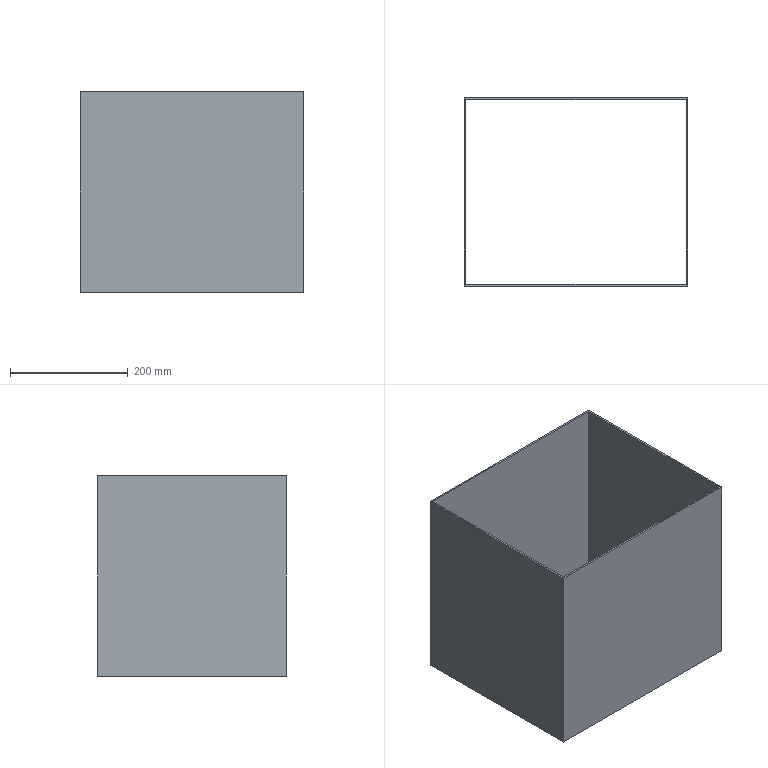Part | SolidWorks | features Extrusion 1 | 1 solid | 10 faces | box 380 x 320 x 340 mm | volume 1415760 mm3 | plane 10
STEP:
#1=CARTESIAN_POINT('',(-190.,160.,170.));
#2=VERTEX_POINT('',#1);
#3=CARTESIAN_POINT('',(-190.,-160.,170.));
#4=VERTEX_POINT('',#3);
#5=CARTESIAN_POINT('',(-190.,160.,170.));
#6=DIRECTION('',(0.,-1.,0.));
#7=VECTOR('',#6,1000.);
#8=LINE('',#5,#7);
#9=EDGE_CURVE('',#2,#4,#8,.T.);
#10=ORIENTED_EDGE('',*,*,#9,.F.);
#11=CARTESIAN_POINT('',(-190.,160.,-170.));
#12=VERTEX_POINT('',#11);
#13=CARTESIAN_POINT('',(-190.,160.,-170.));
#14=DIRECTION('',(0.,0.,1.));
#15=VECTOR('',#14,1000.);
#16=LINE('',#13,#15);
#17=EDGE_CURVE('',#12,#2,#16,.T.);
#18=ORIENTED_EDGE('',*,*,#17,.F.);
#19=CARTESIAN_POINT('',(-190.,-160.,-170.));
#20=VERTEX_POINT('',#19);
#21=CARTESIAN_POINT('',(-190.,160.,-170.));
#22=DIRECTION('',(0.,-1.,0.));
#23=VECTOR('',#22,1000.);
#24=LINE('',#21,#23);
#25=EDGE_CURVE('',#12,#20,#24,.T.);
#26=ORIENTED_EDGE('',*,*,#25,.T.);
#27=CARTESIAN_POINT('',(-190.,-160.,-170.));
#28=DIRECTION('',(0.,0.,1.));
#29=VECTOR('',#28,1000.);
#30=LINE('',#27,#29);
#31=EDGE_CURVE('',#20,#4,#30,.T.);
#32=ORIENTED_EDGE('',*,*,#31,.T.);
#33=EDGE_LOOP('',(#10,#18,#26,#32));
#34=FACE_OUTER_BOUND('',#33,.T.);
#35=CARTESIAN_POINT('',(-190.,160.,-170.));
#36=DIRECTION('',(-1.,0.,0.));
#37=DIRECTION('',(0.,0.,1.));
#38=AXIS2_PLACEMENT_3D('',#35,#36,#37);
#39=PLANE('',#38);
#40=ADVANCED_FACE('',(#34),#39,.T.);
#41=CARTESIAN_POINT('',(190.,160.,170.));
#42=VERTEX_POINT('',#41);
#43=CARTESIAN_POINT('',(190.,160.,170.));
#44=DIRECTION('',(-1.,0.,0.));
#45=VECTOR('',#44,1000.);
#46=LINE('',#43,#45);
#47=EDGE_CURVE('',#42,#2,#46,.T.);
#48=ORIENTED_EDGE('',*,*,#47,.F.);
#49=CARTESIAN_POINT('',(190.,160.,-170.));
#50=VERTEX_POINT('',#49);
#51=CARTESIAN_POINT('',(190.,160.,-170.));
#52=DIRECTION('',(0.,0.,1.));
#53=VECTOR('',#52,1000.);
#54=LINE('',#51,#53);
#55=EDGE_CURVE('',#50,#42,#54,.T.);
#56=ORIENTED_EDGE('',*,*,#55,.F.);
#57=CARTESIAN_POINT('',(190.,160.,-170.));
#58=DIRECTION('',(-1.,0.,0.));
#59=VECTOR('',#58,1000.);
#60=LINE('',#57,#59);
#61=EDGE_CURVE('',#50,#12,#60,.T.);
#62=ORIENTED_EDGE('',*,*,#61,.T.);
#63=ORIENTED_EDGE('',*,*,#17,.T.);
#64=EDGE_LOOP('',(#48,#56,#62,#63));
#65=FACE_OUTER_BOUND('',#64,.T.);
#66=CARTESIAN_POINT('',(190.,160.,-170.));
#67=DIRECTION('',(0.,1.,0.));
#68=DIRECTION('',(0.,0.,1.));
#69=AXIS2_PLACEMENT_3D('',#66,#67,#68);
#70=PLANE('',#69);
#71=ADVANCED_FACE('',(#65),#70,.T.);
#72=CARTESIAN_POINT('',(190.,-160.,170.));
#73=VERTEX_POINT('',#72);
#74=CARTESIAN_POINT('',(190.,-160.,170.));
#75=DIRECTION('',(0.,1.,0.));
#76=VECTOR('',#75,1000.);
#77=LINE('',#74,#76);
#78=EDGE_CURVE('',#73,#42,#77,.T.);
#79=ORIENTED_EDGE('',*,*,#78,.F.);
#80=CARTESIAN_POINT('',(190.,-160.,-170.));
#81=VERTEX_POINT('',#80);
#82=CARTESIAN_POINT('',(190.,-160.,-170.));
#83=DIRECTION('',(0.,0.,1.));
#84=VECTOR('',#83,1000.);
#85=LINE('',#82,#84);
#86=EDGE_CURVE('',#81,#73,#85,.T.);
#87=ORIENTED_EDGE('',*,*,#86,.F.);
#88=CARTESIAN_POINT('',(190.,-160.,-170.));
#89=DIRECTION('',(0.,1.,0.));
#90=VECTOR('',#89,1000.);
#91=LINE('',#88,#90);
#92=EDGE_CURVE('',#81,#50,#91,.T.);
#93=ORIENTED_EDGE('',*,*,#92,.T.);
#94=ORIENTED_EDGE('',*,*,#55,.T.);
#95=EDGE_LOOP('',(#79,#87,#93,#94));
#96=FACE_OUTER_BOUND('',#95,.T.);
#97=CARTESIAN_POINT('',(190.,-160.,-170.));
#98=DIRECTION('',(1.,0.,0.));
#99=DIRECTION('',(0.,0.,-1.));
#100=AXIS2_PLACEMENT_3D('',#97,#98,#99);
#101=PLANE('',#100);
#102=ADVANCED_FACE('',(#96),#101,.T.);
#103=CARTESIAN_POINT('',(-190.,-160.,170.));
#104=DIRECTION('',(1.,0.,0.));
#105=VECTOR('',#104,1000.);
#106=LINE('',#103,#105);
#107=EDGE_CURVE('',#4,#73,#106,.T.);
#108=ORIENTED_EDGE('',*,*,#107,.F.);
#109=ORIENTED_EDGE('',*,*,#31,.F.);
#110=CARTESIAN_POINT('',(-190.,-160.,-170.));
#111=DIRECTION('',(1.,0.,0.));
#112=VECTOR('',#111,1000.);
#113=LINE('',#110,#112);
#114=EDGE_CURVE('',#20,#81,#113,.T.);
#115=ORIENTED_EDGE('',*,*,#114,.T.);
#116=ORIENTED_EDGE('',*,*,#86,.T.);
#117=EDGE_LOOP('',(#108,#109,#115,#116));
#118=FACE_OUTER_BOUND('',#117,.T.);
#119=CARTESIAN_POINT('',(-190.,-160.,-170.));
#120=DIRECTION('',(0.,-1.,0.));
#121=DIRECTION('',(0.,0.,-1.));
#122=AXIS2_PLACEMENT_3D('',#119,#120,#121);
#123=PLANE('',#122);
#124=ADVANCED_FACE('',(#118),#123,.T.);
#125=CARTESIAN_POINT('',(187.,157.,-170.));
#126=VERTEX_POINT('',#125);
#127=CARTESIAN_POINT('',(-187.,157.,-170.));
#128=VERTEX_POINT('',#127);
#129=CARTESIAN_POINT('',(187.,157.,-170.));
#130=DIRECTION('',(-1.,0.,0.));
#131=VECTOR('',#130,1000.);
#132=LINE('',#129,#131);
#133=EDGE_CURVE('',#126,#128,#132,.T.);
#134=ORIENTED_EDGE('',*,*,#133,.T.);
#135=CARTESIAN_POINT('',(-187.,-157.,-170.));
#136=VERTEX_POINT('',#135);
#137=CARTESIAN_POINT('',(-187.,157.,-170.));
#138=DIRECTION('',(0.,-1.,0.));
#139=VECTOR('',#138,1000.);
#140=LINE('',#137,#139);
#141=EDGE_CURVE('',#128,#136,#140,.T.);
#142=ORIENTED_EDGE('',*,*,#141,.T.);
#143=CARTESIAN_POINT('',(187.,-157.,-170.));
#144=VERTEX_POINT('',#143);
#145=CARTESIAN_POINT('',(-187.,-157.,-170.));
#146=DIRECTION('',(1.,0.,0.));
#147=VECTOR('',#146,1000.);
#148=LINE('',#145,#147);
#149=EDGE_CURVE('',#136,#144,#148,.T.);
#150=ORIENTED_EDGE('',*,*,#149,.T.);
#151=CARTESIAN_POINT('',(187.,-157.,-170.));
#152=DIRECTION('',(0.,1.,0.));
#153=VECTOR('',#152,1000.);
#154=LINE('',#151,#153);
#155=EDGE_CURVE('',#144,#126,#154,.T.);
#156=ORIENTED_EDGE('',*,*,#155,.T.);
#157=EDGE_LOOP('',(#134,#142,#150,#156));
#158=FACE_BOUND('',#157,.T.);
#159=ORIENTED_EDGE('',*,*,#25,.F.);
#160=ORIENTED_EDGE('',*,*,#61,.F.);
#161=ORIENTED_EDGE('',*,*,#92,.F.);
#162=ORIENTED_EDGE('',*,*,#114,.F.);
#163=EDGE_LOOP('',(#159,#160,#161,#162));
#164=FACE_OUTER_BOUND('',#163,.T.);
#165=CARTESIAN_POINT('',(0.,0.,-170.));
#166=DIRECTION('',(0.,0.,1.));
#167=DIRECTION('',(1.,0.,0.));
#168=AXIS2_PLACEMENT_3D('',#165,#166,#167);
#169=PLANE('',#168);
#170=ADVANCED_FACE('',(#158,#164),#169,.F.);
#171=CARTESIAN_POINT('',(-187.,157.,170.));
#172=VERTEX_POINT('',#171);
#173=CARTESIAN_POINT('',(-187.,-157.,170.));
#174=VERTEX_POINT('',#173);
#175=CARTESIAN_POINT('',(-187.,157.,170.));
#176=DIRECTION('',(0.,-1.,0.));
#177=VECTOR('',#176,1000.);
#178=LINE('',#175,#177);
#179=EDGE_CURVE('',#172,#174,#178,.T.);
#180=ORIENTED_EDGE('',*,*,#179,.F.);
#181=CARTESIAN_POINT('',(187.,157.,170.));
#182=VERTEX_POINT('',#181);
#183=CARTESIAN_POINT('',(187.,157.,170.));
#184=DIRECTION('',(-1.,0.,0.));
#185=VECTOR('',#184,1000.);
#186=LINE('',#183,#185);
#187=EDGE_CURVE('',#182,#172,#186,.T.);
#188=ORIENTED_EDGE('',*,*,#187,.F.);
#189=CARTESIAN_POINT('',(187.,-157.,170.));
#190=VERTEX_POINT('',#189);
#191=CARTESIAN_POINT('',(187.,-157.,170.));
#192=DIRECTION('',(0.,1.,0.));
#193=VECTOR('',#192,1000.);
#194=LINE('',#191,#193);
#195=EDGE_CURVE('',#190,#182,#194,.T.);
#196=ORIENTED_EDGE('',*,*,#195,.F.);
#197=CARTESIAN_POINT('',(-187.,-157.,170.));
#198=DIRECTION('',(1.,0.,0.));
#199=VECTOR('',#198,1000.);
#200=LINE('',#197,#199);
#201=EDGE_CURVE('',#174,#190,#200,.T.);
#202=ORIENTED_EDGE('',*,*,#201,.F.);
#203=EDGE_LOOP('',(#180,#188,#196,#202));
#204=FACE_BOUND('',#203,.T.);
#205=ORIENTED_EDGE('',*,*,#9,.T.);
#206=ORIENTED_EDGE('',*,*,#107,.T.);
#207=ORIENTED_EDGE('',*,*,#78,.T.);
#208=ORIENTED_EDGE('',*,*,#47,.T.);
#209=EDGE_LOOP('',(#205,#206,#207,#208));
#210=FACE_OUTER_BOUND('',#209,.T.);
#211=CARTESIAN_POINT('',(0.,0.,170.));
#212=DIRECTION('',(0.,0.,1.));
#213=DIRECTION('',(1.,0.,0.));
#214=AXIS2_PLACEMENT_3D('',#211,#212,#213);
#215=PLANE('',#214);
#216=ADVANCED_FACE('',(#204,#210),#215,.T.);
#217=ORIENTED_EDGE('',*,*,#179,.T.);
#218=CARTESIAN_POINT('',(-187.,-157.,-170.));
#219=DIRECTION('',(0.,0.,1.));
#220=VECTOR('',#219,1000.);
#221=LINE('',#218,#220);
#222=EDGE_CURVE('',#136,#174,#221,.T.);
#223=ORIENTED_EDGE('',*,*,#222,.F.);
#224=ORIENTED_EDGE('',*,*,#141,.F.);
#225=CARTESIAN_POINT('',(-187.,157.,-170.));
#226=DIRECTION('',(0.,0.,1.));
#227=VECTOR('',#226,1000.);
#228=LINE('',#225,#227);
#229=EDGE_CURVE('',#128,#172,#228,.T.);
#230=ORIENTED_EDGE('',*,*,#229,.T.);
#231=EDGE_LOOP('',(#217,#223,#224,#230));
#232=FACE_OUTER_BOUND('',#231,.T.);
#233=CARTESIAN_POINT('',(-187.,157.,-170.));
#234=DIRECTION('',(-1.,0.,0.));
#235=DIRECTION('',(0.,0.,1.));
#236=AXIS2_PLACEMENT_3D('',#233,#234,#235);
#237=PLANE('',#236);
#238=ADVANCED_FACE('',(#232),#237,.F.);
#239=ORIENTED_EDGE('',*,*,#187,.T.);
#240=ORIENTED_EDGE('',*,*,#229,.F.);
#241=ORIENTED_EDGE('',*,*,#133,.F.);
#242=CARTESIAN_POINT('',(187.,157.,-170.));
#243=DIRECTION('',(0.,0.,1.));
#244=VECTOR('',#243,1000.);
#245=LINE('',#242,#244);
#246=EDGE_CURVE('',#126,#182,#245,.T.);
#247=ORIENTED_EDGE('',*,*,#246,.T.);
#248=EDGE_LOOP('',(#239,#240,#241,#247));
#249=FACE_OUTER_BOUND('',#248,.T.);
#250=CARTESIAN_POINT('',(187.,157.,-170.));
#251=DIRECTION('',(0.,1.,0.));
#252=DIRECTION('',(0.,0.,1.));
#253=AXIS2_PLACEMENT_3D('',#250,#251,#252);
#254=PLANE('',#253);
#255=ADVANCED_FACE('',(#249),#254,.F.);
#256=ORIENTED_EDGE('',*,*,#195,.T.);
#257=ORIENTED_EDGE('',*,*,#246,.F.);
#258=ORIENTED_EDGE('',*,*,#155,.F.);
#259=CARTESIAN_POINT('',(187.,-157.,-170.));
#260=DIRECTION('',(0.,0.,1.));
#261=VECTOR('',#260,1000.);
#262=LINE('',#259,#261);
#263=EDGE_CURVE('',#144,#190,#262,.T.);
#264=ORIENTED_EDGE('',*,*,#263,.T.);
#265=EDGE_LOOP('',(#256,#257,#258,#264));
#266=FACE_OUTER_BOUND('',#265,.T.);
#267=CARTESIAN_POINT('',(187.,-157.,-170.));
#268=DIRECTION('',(1.,0.,0.));
#269=DIRECTION('',(0.,0.,-1.));
#270=AXIS2_PLACEMENT_3D('',#267,#268,#269);
#271=PLANE('',#270);
#272=ADVANCED_FACE('',(#266),#271,.F.);
#273=ORIENTED_EDGE('',*,*,#201,.T.);
#274=ORIENTED_EDGE('',*,*,#263,.F.);
#275=ORIENTED_EDGE('',*,*,#149,.F.);
#276=ORIENTED_EDGE('',*,*,#222,.T.);
#277=EDGE_LOOP('',(#273,#274,#275,#276));
#278=FACE_OUTER_BOUND('',#277,.T.);
#279=CARTESIAN_POINT('',(-187.,-157.,-170.));
#280=DIRECTION('',(0.,-1.,0.));
#281=DIRECTION('',(0.,0.,-1.));
#282=AXIS2_PLACEMENT_3D('',#279,#280,#281);
#283=PLANE('',#282);
#284=ADVANCED_FACE('',(#278),#283,.F.);
#285=CLOSED_SHELL('',(#40,#71,#102,#124,#170,#216,#238,#255,#272,#284));
#286=MANIFOLD_SOLID_BREP('',#285);
#287=CARTESIAN_POINT('',(0.,0.,0.));
#288=DIRECTION('',(0.,0.,1.));
#289=DIRECTION('',(1.,0.,0.));
#290=AXIS2_PLACEMENT_3D('',#287,#288,#289);
#291=(LENGTH_UNIT()NAMED_UNIT(*)SI_UNIT(.MILLI.,.METRE.));
#292=UNCERTAINTY_MEASURE_WITH_UNIT(LENGTH_MEASURE(0.00001),#291,'','');
#293=(NAMED_UNIT(*)PLANE_ANGLE_UNIT()SI_UNIT($,.RADIAN.));
#294=(NAMED_UNIT(*)SI_UNIT($,.STERADIAN.)SOLID_ANGLE_UNIT());
#295=(GEOMETRIC_REPRESENTATION_CONTEXT(3)GLOBAL_UNCERTAINTY_ASSIGNED_CONTEXT((#292))GLOBAL_UNIT_ASSIGNED_CONTEXT((#291,#293,#294))REPRESENTATION_CONTEXT('',''));
#296=ADVANCED_BREP_SHAPE_REPRESENTATION('',(#286,#290),#295);